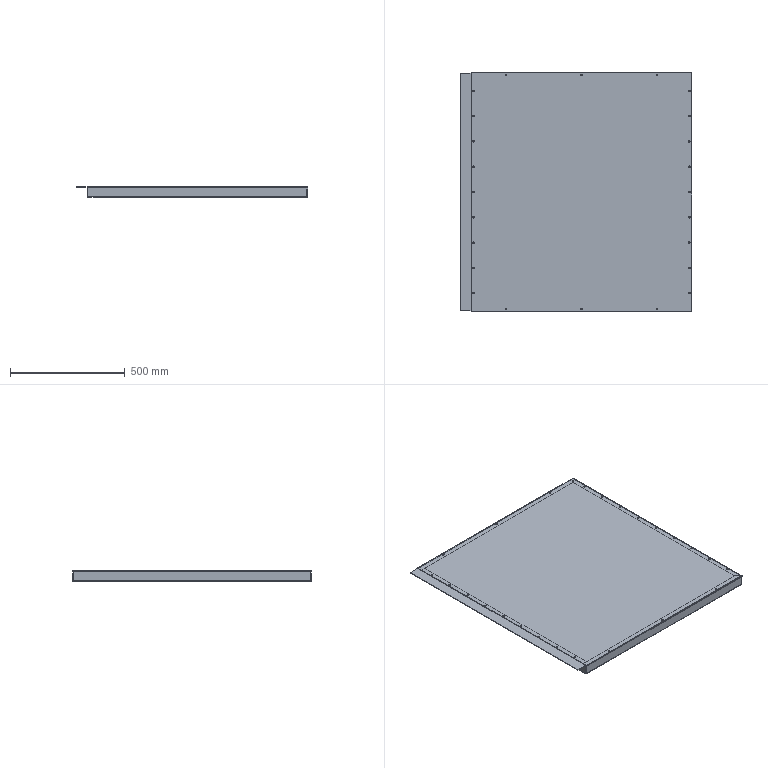Part | SolidWorks | 3 solids | 178 faces | box 1010 x 1043 x 48 mm | volume 5239556 mm3 | cylinder 112 | plane 54 | spline 12 | commonest cylinder face diameters 5 x48 6.5 x48 1.473 x8 6.473 x8